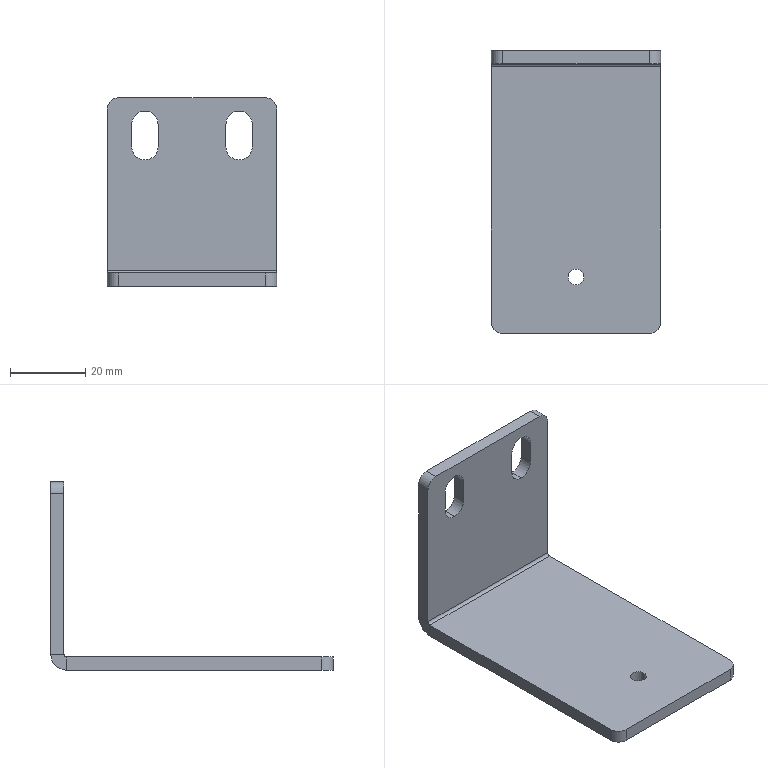Part | SolidWorks | features HoleWzd 2, EdgeFlange 1, Fillet 1, FlatPattern 1, ICE 1, MirrorPattern 1, SMBaseFlange 1, SheetMetal 1 | 1 solid | 30 faces | box 45 x 75 x 50 mm | volume 18329 mm3 | plane 16 | cylinder 14 | commonest cylinder face diameters 7 x6 6 x4 4.2 x2 1.473 x1 8.473 x1
STEP:
#1=CARTESIAN_POINT('',(16.,37.5,33.5));
#2=VERTEX_POINT('',#1);
#3=CARTESIAN_POINT('',(12.5,37.5,30.));
#4=VERTEX_POINT('',#3);
#5=CARTESIAN_POINT('',(12.5,37.5,33.5));
#6=DIRECTION('',(0.,1.,0.));
#7=DIRECTION('',(0.,0.,-1.));
#8=AXIS2_PLACEMENT_3D('',#5,#6,#7);
#9=CIRCLE('',#8,3.5);
#10=EDGE_CURVE('',#2,#4,#9,.T.);
#11=ORIENTED_EDGE('',*,*,#10,.T.);
#12=CARTESIAN_POINT('',(12.5,34.,30.));
#13=VERTEX_POINT('',#12);
#14=CARTESIAN_POINT('',(12.5,37.5,30.));
#15=DIRECTION('',(0.,-1.,0.));
#16=VECTOR('',#15,1000.);
#17=LINE('',#14,#16);
#18=EDGE_CURVE('',#4,#13,#17,.T.);
#19=ORIENTED_EDGE('',*,*,#18,.T.);
#20=CARTESIAN_POINT('',(16.,34.,33.5));
#21=VERTEX_POINT('',#20);
#22=CARTESIAN_POINT('',(12.5,34.,33.5));
#23=DIRECTION('',(0.,1.,0.));
#24=DIRECTION('',(0.,0.,-1.));
#25=AXIS2_PLACEMENT_3D('',#22,#23,#24);
#26=CIRCLE('',#25,3.5);
#27=EDGE_CURVE('',#21,#13,#26,.T.);
#28=ORIENTED_EDGE('',*,*,#27,.F.);
#29=CARTESIAN_POINT('',(16.,37.5,33.5));
#30=DIRECTION('',(0.,-1.,0.));
#31=VECTOR('',#30,1000.);
#32=LINE('',#29,#31);
#33=EDGE_CURVE('',#2,#21,#32,.T.);
#34=ORIENTED_EDGE('',*,*,#33,.F.);
#35=EDGE_LOOP('',(#11,#19,#28,#34));
#36=FACE_OUTER_BOUND('',#35,.T.);
#37=CARTESIAN_POINT('',(12.5,37.5,33.5));
#38=DIRECTION('',(0.,-1.,0.));
#39=DIRECTION('',(0.,0.,-1.));
#40=AXIS2_PLACEMENT_3D('',#37,#38,#39);
#41=CYLINDRICAL_SURFACE('',#40,3.5);
#42=ADVANCED_FACE('',(#36),#41,.F.);
#43=CARTESIAN_POINT('',(-12.5,37.5,30.));
#44=VERTEX_POINT('',#43);
#45=CARTESIAN_POINT('',(-9.,37.5,33.5));
#46=VERTEX_POINT('',#45);
#47=CARTESIAN_POINT('',(-12.5,37.5,33.5));
#48=DIRECTION('',(0.,-1.,0.));
#49=DIRECTION('',(0.,0.,-1.));
#50=AXIS2_PLACEMENT_3D('',#47,#48,#49);
#51=CIRCLE('',#50,3.5);
#52=EDGE_CURVE('',#44,#46,#51,.T.);
#53=ORIENTED_EDGE('',*,*,#52,.F.);
#54=CARTESIAN_POINT('',(-12.5,34.,30.));
#55=VERTEX_POINT('',#54);
#56=CARTESIAN_POINT('',(-12.5,37.5,30.));
#57=DIRECTION('',(0.,-1.,0.));
#58=VECTOR('',#57,1000.);
#59=LINE('',#56,#58);
#60=EDGE_CURVE('',#44,#55,#59,.T.);
#61=ORIENTED_EDGE('',*,*,#60,.T.);
#62=CARTESIAN_POINT('',(-9.,34.,33.5));
#63=VERTEX_POINT('',#62);
#64=CARTESIAN_POINT('',(-12.5,34.,33.5));
#65=DIRECTION('',(0.,-1.,0.));
#66=DIRECTION('',(0.,0.,-1.));
#67=AXIS2_PLACEMENT_3D('',#64,#65,#66);
#68=CIRCLE('',#67,3.5);
#69=EDGE_CURVE('',#55,#63,#68,.T.);
#70=ORIENTED_EDGE('',*,*,#69,.T.);
#71=CARTESIAN_POINT('',(-9.,37.5,33.5));
#72=DIRECTION('',(0.,-1.,0.));
#73=VECTOR('',#72,1000.);
#74=LINE('',#71,#73);
#75=EDGE_CURVE('',#46,#63,#74,.T.);
#76=ORIENTED_EDGE('',*,*,#75,.F.);
#77=EDGE_LOOP('',(#53,#61,#70,#76));
#78=FACE_OUTER_BOUND('',#77,.T.);
#79=CARTESIAN_POINT('',(-12.5,37.5,33.5));
#80=DIRECTION('',(0.,-1.,0.));
#81=DIRECTION('',(0.,0.,-1.));
#82=AXIS2_PLACEMENT_3D('',#79,#80,#81);
#83=CYLINDRICAL_SURFACE('',#82,3.5);
#84=ADVANCED_FACE('',(#78),#83,.F.);
#85=CARTESIAN_POINT('',(-2.1,-22.5,-3.5));
#86=VERTEX_POINT('',#85);
#87=CARTESIAN_POINT('',(2.1,-22.5,-3.5));
#88=VERTEX_POINT('',#87);
#89=CARTESIAN_POINT('',(0.,-22.5,-3.5));
#90=DIRECTION('',(0.,0.,1.));
#91=DIRECTION('',(1.,0.,0.));
#92=AXIS2_PLACEMENT_3D('',#89,#90,#91);
#93=CIRCLE('',#92,2.1);
#94=EDGE_CURVE('',#86,#88,#93,.T.);
#95=ORIENTED_EDGE('',*,*,#94,.F.);
#96=CARTESIAN_POINT('',(-2.1,-22.5,0.));
#97=VERTEX_POINT('',#96);
#98=CARTESIAN_POINT('',(-2.1,-22.5,0.));
#99=DIRECTION('',(0.,0.,1.));
#100=VECTOR('',#99,1000.);
#101=LINE('',#98,#100);
#102=EDGE_CURVE('',#86,#97,#101,.T.);
#103=ORIENTED_EDGE('',*,*,#102,.T.);
#104=CARTESIAN_POINT('',(2.1,-22.5,0.));
#105=VERTEX_POINT('',#104);
#106=CARTESIAN_POINT('',(0.,-22.5,0.));
#107=DIRECTION('',(0.,0.,1.));
#108=DIRECTION('',(1.,0.,0.));
#109=AXIS2_PLACEMENT_3D('',#106,#107,#108);
#110=CIRCLE('',#109,2.1);
#111=EDGE_CURVE('',#97,#105,#110,.T.);
#112=ORIENTED_EDGE('',*,*,#111,.T.);
#113=CARTESIAN_POINT('',(2.1,-22.5,0.));
#114=DIRECTION('',(0.,0.,1.));
#115=VECTOR('',#114,1000.);
#116=LINE('',#113,#115);
#117=EDGE_CURVE('',#88,#105,#116,.T.);
#118=ORIENTED_EDGE('',*,*,#117,.F.);
#119=EDGE_LOOP('',(#95,#103,#112,#118));
#120=FACE_OUTER_BOUND('',#119,.T.);
#121=CARTESIAN_POINT('',(0.,-22.5,0.));
#122=DIRECTION('',(0.,0.,1.));
#123=DIRECTION('',(1.,0.,0.));
#124=AXIS2_PLACEMENT_3D('',#121,#122,#123);
#125=CYLINDRICAL_SURFACE('',#124,2.1);
#126=ADVANCED_FACE('',(#120),#125,.F.);
#127=CARTESIAN_POINT('',(-16.,37.5,33.5));
#128=VERTEX_POINT('',#127);
#129=CARTESIAN_POINT('',(-12.5,37.5,33.5));
#130=DIRECTION('',(0.,-1.,0.));
#131=DIRECTION('',(0.,0.,-1.));
#132=AXIS2_PLACEMENT_3D('',#129,#130,#131);
#133=CIRCLE('',#132,3.5);
#134=EDGE_CURVE('',#128,#44,#133,.T.);
#135=ORIENTED_EDGE('',*,*,#134,.T.);
#136=ORIENTED_EDGE('',*,*,#52,.T.);
#137=CARTESIAN_POINT('',(-9.,37.5,39.5));
#138=VERTEX_POINT('',#137);
#139=CARTESIAN_POINT('',(-9.,37.5,39.5));
#140=DIRECTION('',(0.,0.,1.));
#141=VECTOR('',#140,1000.);
#142=LINE('',#139,#141);
#143=EDGE_CURVE('',#46,#138,#142,.T.);
#144=ORIENTED_EDGE('',*,*,#143,.T.);
#145=CARTESIAN_POINT('',(-16.,37.5,39.5));
#146=VERTEX_POINT('',#145);
#147=CARTESIAN_POINT('',(-12.5,37.5,39.5));
#148=DIRECTION('',(0.,-1.,0.));
#149=DIRECTION('',(0.,0.,-1.));
#150=AXIS2_PLACEMENT_3D('',#147,#148,#149);
#151=CIRCLE('',#150,3.5);
#152=EDGE_CURVE('',#138,#146,#151,.T.);
#153=ORIENTED_EDGE('',*,*,#152,.T.);
#154=CARTESIAN_POINT('',(-16.,37.5,39.5));
#155=DIRECTION('',(0.,0.,-1.));
#156=VECTOR('',#155,1000.);
#157=LINE('',#154,#156);
#158=EDGE_CURVE('',#146,#128,#157,.T.);
#159=ORIENTED_EDGE('',*,*,#158,.T.);
#160=EDGE_LOOP('',(#135,#136,#144,#153,#159));
#161=FACE_BOUND('',#160,.T.);
#162=CARTESIAN_POINT('',(-19.5,37.5,46.5));
#163=VERTEX_POINT('',#162);
#164=CARTESIAN_POINT('',(19.5,37.5,46.5));
#165=VERTEX_POINT('',#164);
#166=CARTESIAN_POINT('',(0.,37.5,46.5));
#167=DIRECTION('',(1.,0.,0.));
#168=VECTOR('',#167,1000.);
#169=LINE('',#166,#168);
#170=EDGE_CURVE('',#163,#165,#169,.T.);
#171=ORIENTED_EDGE('',*,*,#170,.T.);
#172=CARTESIAN_POINT('',(22.5,37.5,43.5));
#173=VERTEX_POINT('',#172);
#174=CARTESIAN_POINT('',(19.5,37.5,43.5));
#175=DIRECTION('',(0.,1.,0.));
#176=DIRECTION('',(0.,0.,-1.));
#177=AXIS2_PLACEMENT_3D('',#174,#175,#176);
#178=CIRCLE('',#177,3.);
#179=EDGE_CURVE('',#165,#173,#178,.T.);
#180=ORIENTED_EDGE('',*,*,#179,.T.);
#181=CARTESIAN_POINT('',(22.5,37.5,0.7366));
#182=VERTEX_POINT('',#181);
#183=CARTESIAN_POINT('',(22.5,37.5,0.));
#184=DIRECTION('',(0.,0.,-1.));
#185=VECTOR('',#184,1000.);
#186=LINE('',#183,#185);
#187=EDGE_CURVE('',#173,#182,#186,.T.);
#188=ORIENTED_EDGE('',*,*,#187,.T.);
#189=CARTESIAN_POINT('',(-22.5,37.5,0.7366));
#190=VERTEX_POINT('',#189);
#191=CARTESIAN_POINT('',(22.5,37.5,0.7366));
#192=DIRECTION('',(1.,0.,0.));
#193=VECTOR('',#192,1000.);
#194=LINE('',#191,#193);
#195=EDGE_CURVE('',#190,#182,#194,.T.);
#196=ORIENTED_EDGE('',*,*,#195,.F.);
#197=CARTESIAN_POINT('',(-22.5,37.5,43.5));
#198=VERTEX_POINT('',#197);
#199=CARTESIAN_POINT('',(-22.5,37.5,0.));
#200=DIRECTION('',(0.,0.,1.));
#201=VECTOR('',#200,1000.);
#202=LINE('',#199,#201);
#203=EDGE_CURVE('',#190,#198,#202,.T.);
#204=ORIENTED_EDGE('',*,*,#203,.T.);
#205=CARTESIAN_POINT('',(-19.5,37.5,43.5));
#206=DIRECTION('',(0.,1.,0.));
#207=DIRECTION('',(0.,0.,-1.));
#208=AXIS2_PLACEMENT_3D('',#205,#206,#207);
#209=CIRCLE('',#208,3.);
#210=EDGE_CURVE('',#198,#163,#209,.T.);
#211=ORIENTED_EDGE('',*,*,#210,.T.);
#212=EDGE_LOOP('',(#171,#180,#188,#196,#204,#211));
#213=FACE_OUTER_BOUND('',#212,.T.);
#214=CARTESIAN_POINT('',(9.,37.5,39.5));
#215=VERTEX_POINT('',#214);
#216=CARTESIAN_POINT('',(16.,37.5,39.5));
#217=VERTEX_POINT('',#216);
#218=CARTESIAN_POINT('',(12.5,37.5,39.5));
#219=DIRECTION('',(0.,1.,0.));
#220=DIRECTION('',(0.,0.,-1.));
#221=AXIS2_PLACEMENT_3D('',#218,#219,#220);
#222=CIRCLE('',#221,3.5);
#223=EDGE_CURVE('',#215,#217,#222,.T.);
#224=ORIENTED_EDGE('',*,*,#223,.F.);
#225=CARTESIAN_POINT('',(9.,37.5,33.5));
#226=VERTEX_POINT('',#225);
#227=CARTESIAN_POINT('',(9.,37.5,39.5));
#228=DIRECTION('',(0.,0.,1.));
#229=VECTOR('',#228,1000.);
#230=LINE('',#227,#229);
#231=EDGE_CURVE('',#226,#215,#230,.T.);
#232=ORIENTED_EDGE('',*,*,#231,.F.);
#233=CARTESIAN_POINT('',(12.5,37.5,33.5));
#234=DIRECTION('',(0.,1.,0.));
#235=DIRECTION('',(0.,0.,-1.));
#236=AXIS2_PLACEMENT_3D('',#233,#234,#235);
#237=CIRCLE('',#236,3.5);
#238=EDGE_CURVE('',#4,#226,#237,.T.);
#239=ORIENTED_EDGE('',*,*,#238,.F.);
#240=ORIENTED_EDGE('',*,*,#10,.F.);
#241=CARTESIAN_POINT('',(16.,37.5,39.5));
#242=DIRECTION('',(0.,0.,-1.));
#243=VECTOR('',#242,1000.);
#244=LINE('',#241,#243);
#245=EDGE_CURVE('',#217,#2,#244,.T.);
#246=ORIENTED_EDGE('',*,*,#245,.F.);
#247=EDGE_LOOP('',(#224,#232,#239,#240,#246));
#248=FACE_BOUND('',#247,.T.);
#249=CARTESIAN_POINT('',(0.,37.5,0.));
#250=DIRECTION('',(0.,-1.,0.));
#251=DIRECTION('',(0.,0.,-1.));
#252=AXIS2_PLACEMENT_3D('',#249,#250,#251);
#253=PLANE('',#252);
#254=ADVANCED_FACE('',(#161,#213,#248),#253,.F.);
#255=CARTESIAN_POINT('',(-9.,34.,39.5));
#256=VERTEX_POINT('',#255);
#257=CARTESIAN_POINT('',(-9.,34.,39.5));
#258=DIRECTION('',(0.,0.,1.));
#259=VECTOR('',#258,1000.);
#260=LINE('',#257,#259);
#261=EDGE_CURVE('',#63,#256,#260,.T.);
#262=ORIENTED_EDGE('',*,*,#261,.F.);
#263=ORIENTED_EDGE('',*,*,#69,.F.);
#264=CARTESIAN_POINT('',(-16.,34.,33.5));
#265=VERTEX_POINT('',#264);
#266=CARTESIAN_POINT('',(-12.5,34.,33.5));
#267=DIRECTION('',(0.,-1.,0.));
#268=DIRECTION('',(0.,0.,-1.));
#269=AXIS2_PLACEMENT_3D('',#266,#267,#268);
#270=CIRCLE('',#269,3.5);
#271=EDGE_CURVE('',#265,#55,#270,.T.);
#272=ORIENTED_EDGE('',*,*,#271,.F.);
#273=CARTESIAN_POINT('',(-16.,34.,39.5));
#274=VERTEX_POINT('',#273);
#275=CARTESIAN_POINT('',(-16.,34.,39.5));
#276=DIRECTION('',(0.,0.,-1.));
#277=VECTOR('',#276,1000.);
#278=LINE('',#275,#277);
#279=EDGE_CURVE('',#274,#265,#278,.T.);
#280=ORIENTED_EDGE('',*,*,#279,.F.);
#281=CARTESIAN_POINT('',(-12.5,34.,39.5));
#282=DIRECTION('',(0.,-1.,0.));
#283=DIRECTION('',(0.,0.,-1.));
#284=AXIS2_PLACEMENT_3D('',#281,#282,#283);
#285=CIRCLE('',#284,3.5);
#286=EDGE_CURVE('',#256,#274,#285,.T.);
#287=ORIENTED_EDGE('',*,*,#286,.F.);
#288=EDGE_LOOP('',(#262,#263,#272,#280,#287));
#289=FACE_BOUND('',#288,.T.);
#290=CARTESIAN_POINT('',(22.5,34.,43.5));
#291=VERTEX_POINT('',#290);
#292=CARTESIAN_POINT('',(22.5,34.,0.7366));
#293=VERTEX_POINT('',#292);
#294=CARTESIAN_POINT('',(22.5,34.,0.));
#295=DIRECTION('',(0.,0.,-1.));
#296=VECTOR('',#295,1000.);
#297=LINE('',#294,#296);
#298=EDGE_CURVE('',#291,#293,#297,.T.);
#299=ORIENTED_EDGE('',*,*,#298,.F.);
#300=CARTESIAN_POINT('',(19.5,34.,46.5));
#301=VERTEX_POINT('',#300);
#302=CARTESIAN_POINT('',(19.5,34.,43.5));
#303=DIRECTION('',(0.,-1.,0.));
#304=DIRECTION('',(0.,0.,-1.));
#305=AXIS2_PLACEMENT_3D('',#302,#303,#304);
#306=CIRCLE('',#305,3.);
#307=EDGE_CURVE('',#291,#301,#306,.T.);
#308=ORIENTED_EDGE('',*,*,#307,.T.);
#309=CARTESIAN_POINT('',(-19.5,34.,46.5));
#310=VERTEX_POINT('',#309);
#311=CARTESIAN_POINT('',(22.5,34.,46.5));
#312=DIRECTION('',(1.,0.,0.));
#313=VECTOR('',#312,1000.);
#314=LINE('',#311,#313);
#315=EDGE_CURVE('',#310,#301,#314,.T.);
#316=ORIENTED_EDGE('',*,*,#315,.F.);
#317=CARTESIAN_POINT('',(-22.5,34.,43.5));
#318=VERTEX_POINT('',#317);
#319=CARTESIAN_POINT('',(-19.5,34.,43.5));
#320=DIRECTION('',(0.,-1.,0.));
#321=DIRECTION('',(0.,0.,-1.));
#322=AXIS2_PLACEMENT_3D('',#319,#320,#321);
#323=CIRCLE('',#322,3.);
#324=EDGE_CURVE('',#310,#318,#323,.T.);
#325=ORIENTED_EDGE('',*,*,#324,.T.);
#326=CARTESIAN_POINT('',(-22.5,34.,0.7366));
#327=VERTEX_POINT('',#326);
#328=CARTESIAN_POINT('',(-22.5,34.,46.5));
#329=DIRECTION('',(0.,0.,1.));
#330=VECTOR('',#329,1000.);
#331=LINE('',#328,#330);
#332=EDGE_CURVE('',#327,#318,#331,.T.);
#333=ORIENTED_EDGE('',*,*,#332,.F.);
#334=CARTESIAN_POINT('',(22.5,34.,0.7366));
#335=DIRECTION('',(-1.,0.,0.));
#336=VECTOR('',#335,1000.);
#337=LINE('',#334,#336);
#338=EDGE_CURVE('',#293,#327,#337,.T.);
#339=ORIENTED_EDGE('',*,*,#338,.F.);
#340=EDGE_LOOP('',(#299,#308,#316,#325,#333,#339));
#341=FACE_OUTER_BOUND('',#340,.T.);
#342=CARTESIAN_POINT('',(9.,34.,33.5));
#343=VERTEX_POINT('',#342);
#344=CARTESIAN_POINT('',(9.,34.,39.5));
#345=VERTEX_POINT('',#344);
#346=CARTESIAN_POINT('',(9.,34.,39.5));
#347=DIRECTION('',(0.,0.,1.));
#348=VECTOR('',#347,1000.);
#349=LINE('',#346,#348);
#350=EDGE_CURVE('',#343,#345,#349,.T.);
#351=ORIENTED_EDGE('',*,*,#350,.T.);
#352=CARTESIAN_POINT('',(16.,34.,39.5));
#353=VERTEX_POINT('',#352);
#354=CARTESIAN_POINT('',(12.5,34.,39.5));
#355=DIRECTION('',(0.,1.,0.));
#356=DIRECTION('',(0.,0.,-1.));
#357=AXIS2_PLACEMENT_3D('',#354,#355,#356);
#358=CIRCLE('',#357,3.5);
#359=EDGE_CURVE('',#345,#353,#358,.T.);
#360=ORIENTED_EDGE('',*,*,#359,.T.);
#361=CARTESIAN_POINT('',(16.,34.,39.5));
#362=DIRECTION('',(0.,0.,-1.));
#363=VECTOR('',#362,1000.);
#364=LINE('',#361,#363);
#365=EDGE_CURVE('',#353,#21,#364,.T.);
#366=ORIENTED_EDGE('',*,*,#365,.T.);
#367=ORIENTED_EDGE('',*,*,#27,.T.);
#368=CARTESIAN_POINT('',(12.5,34.,33.5));
#369=DIRECTION('',(0.,1.,0.));
#370=DIRECTION('',(0.,0.,-1.));
#371=AXIS2_PLACEMENT_3D('',#368,#369,#370);
#372=CIRCLE('',#371,3.5);
#373=EDGE_CURVE('',#13,#343,#372,.T.);
#374=ORIENTED_EDGE('',*,*,#373,.T.);
#375=EDGE_LOOP('',(#351,#360,#366,#367,#374));
#376=FACE_BOUND('',#375,.T.);
#377=CARTESIAN_POINT('',(0.,34.,0.));
#378=DIRECTION('',(0.,-1.,0.));
#379=DIRECTION('',(0.,0.,-1.));
#380=AXIS2_PLACEMENT_3D('',#377,#378,#379);
#381=PLANE('',#380);
#382=ADVANCED_FACE('',(#289,#341,#376),#381,.T.);
#383=CARTESIAN_POINT('',(-22.5,33.263,-3.5));
#384=VERTEX_POINT('',#383);
#385=CARTESIAN_POINT('',(-22.5,-34.5,-3.5));
#386=VERTEX_POINT('',#385);
#387=CARTESIAN_POINT('',(-22.5,37.5,-3.5));
#388=DIRECTION('',(0.,-1.,0.));
#389=VECTOR('',#388,1000.);
#390=LINE('',#387,#389);
#391=EDGE_CURVE('',#384,#386,#390,.T.);
#392=ORIENTED_EDGE('',*,*,#391,.T.);
#393=CARTESIAN_POINT('',(-22.5,-34.5,0.));
#394=VERTEX_POINT('',#393);
#395=CARTESIAN_POINT('',(-22.5,-34.5,-3.5));
#396=DIRECTION('',(0.,0.,1.));
#397=VECTOR('',#396,1000.);
#398=LINE('',#395,#397);
#399=EDGE_CURVE('',#386,#394,#398,.T.);
#400=ORIENTED_EDGE('',*,*,#399,.T.);
#401=CARTESIAN_POINT('',(-22.5,33.263,0.));
#402=VERTEX_POINT('',#401);
#403=CARTESIAN_POINT('',(-22.5,37.5,0.));
#404=DIRECTION('',(0.,-1.,0.));
#405=VECTOR('',#404,1000.);
#406=LINE('',#403,#405);
#407=EDGE_CURVE('',#402,#394,#406,.T.);
#408=ORIENTED_EDGE('',*,*,#407,.F.);
#409=CARTESIAN_POINT('',(-22.5,33.263,0.));
#410=DIRECTION('',(0.,0.,-1.));
#411=VECTOR('',#410,1000.);
#412=LINE('',#409,#411);
#413=EDGE_CURVE('',#402,#384,#412,.T.);
#414=ORIENTED_EDGE('',*,*,#413,.T.);
#415=EDGE_LOOP('',(#392,#400,#408,#414));
#416=FACE_OUTER_BOUND('',#415,.T.);
#417=CARTESIAN_POINT('',(-22.5,37.5,-3.5));
#418=DIRECTION('',(-1.,0.,0.));
#419=DIRECTION('',(0.,-1.,0.));
#420=AXIS2_PLACEMENT_3D('',#417,#418,#419);
#421=PLANE('',#420);
#422=ADVANCED_FACE('',(#416),#421,.T.);
#423=CARTESIAN_POINT('',(0.,-22.5,-3.5));
#424=DIRECTION('',(0.,0.,1.));
#425=DIRECTION('',(1.,0.,0.));
#426=AXIS2_PLACEMENT_3D('',#423,#424,#425);
#427=CIRCLE('',#426,2.1);
#428=EDGE_CURVE('',#88,#86,#427,.T.);
#429=ORIENTED_EDGE('',*,*,#428,.T.);
#430=ORIENTED_EDGE('',*,*,#94,.T.);
#431=EDGE_LOOP('',(#429,#430));
#432=FACE_BOUND('',#431,.T.);
#433=CARTESIAN_POINT('',(-19.5,-37.5,-3.5));
#434=VERTEX_POINT('',#433);
#435=CARTESIAN_POINT('',(19.5,-37.5,-3.5));
#436=VERTEX_POINT('',#435);
#437=CARTESIAN_POINT('',(-22.5,-37.5,-3.5));
#438=DIRECTION('',(1.,0.,0.));
#439=VECTOR('',#438,1000.);
#440=LINE('',#437,#439);
#441=EDGE_CURVE('',#434,#436,#440,.T.);
#442=ORIENTED_EDGE('',*,*,#441,.F.);
#443=CARTESIAN_POINT('',(-19.5,-34.5,-3.5));
#444=DIRECTION('',(0.,0.,-1.));
#445=DIRECTION('',(1.,0.,0.));
#446=AXIS2_PLACEMENT_3D('',#443,#444,#445);
#447=CIRCLE('',#446,3.);
#448=EDGE_CURVE('',#434,#386,#447,.T.);
#449=ORIENTED_EDGE('',*,*,#448,.T.);
#450=ORIENTED_EDGE('',*,*,#391,.F.);
#451=CARTESIAN_POINT('',(22.5,33.263,-3.5));
#452=VERTEX_POINT('',#451);
#453=CARTESIAN_POINT('',(-22.5,33.263,-3.5));
#454=DIRECTION('',(1.,0.,0.));
#455=VECTOR('',#454,1000.);
#456=LINE('',#453,#455);
#457=EDGE_CURVE('',#384,#452,#456,.T.);
#458=ORIENTED_EDGE('',*,*,#457,.T.);
#459=CARTESIAN_POINT('',(22.5,-34.5,-3.5));
#460=VERTEX_POINT('',#459);
#461=CARTESIAN_POINT('',(22.5,37.5,-3.5));
#462=DIRECTION('',(0.,1.,0.));
#463=VECTOR('',#462,1000.);
#464=LINE('',#461,#463);
#465=EDGE_CURVE('',#460,#452,#464,.T.);
#466=ORIENTED_EDGE('',*,*,#465,.F.);
#467=CARTESIAN_POINT('',(19.5,-34.5,-3.5));
#468=DIRECTION('',(0.,0.,-1.));
#469=DIRECTION('',(1.,0.,0.));
#470=AXIS2_PLACEMENT_3D('',#467,#468,#469);
#471=CIRCLE('',#470,3.);
#472=EDGE_CURVE('',#460,#436,#471,.T.);
#473=ORIENTED_EDGE('',*,*,#472,.T.);
#474=EDGE_LOOP('',(#442,#449,#450,#458,#466,#473));
#475=FACE_OUTER_BOUND('',#474,.T.);
#476=CARTESIAN_POINT('',(0.,0.,-3.5));
#477=DIRECTION('',(0.,0.,1.));
#478=DIRECTION('',(1.,0.,0.));
#479=AXIS2_PLACEMENT_3D('',#476,#477,#478);
#480=PLANE('',#479);
#481=ADVANCED_FACE('',(#432,#475),#480,.F.);
#482=CARTESIAN_POINT('',(0.,-22.5,0.));
#483=DIRECTION('',(0.,0.,1.));
#484=DIRECTION('',(1.,0.,0.));
#485=AXIS2_PLACEMENT_3D('',#482,#483,#484);
#486=CIRCLE('',#485,2.1);
#487=EDGE_CURVE('',#105,#97,#486,.T.);
#488=ORIENTED_EDGE('',*,*,#487,.F.);
#489=ORIENTED_EDGE('',*,*,#111,.F.);
#490=EDGE_LOOP('',(#488,#489));
#491=FACE_BOUND('',#490,.T.);
#492=ORIENTED_EDGE('',*,*,#407,.T.);
#493=CARTESIAN_POINT('',(-19.5,-37.5,0.));
#494=VERTEX_POINT('',#493);
#495=CARTESIAN_POINT('',(-19.5,-34.5,0.));
#496=DIRECTION('',(0.,0.,1.));
#497=DIRECTION('',(1.,0.,0.));
#498=AXIS2_PLACEMENT_3D('',#495,#496,#497);
#499=CIRCLE('',#498,3.);
#500=EDGE_CURVE('',#394,#494,#499,.T.);
#501=ORIENTED_EDGE('',*,*,#500,.T.);
#502=CARTESIAN_POINT('',(19.5,-37.5,0.));
#503=VERTEX_POINT('',#502);
#504=CARTESIAN_POINT('',(-22.5,-37.5,0.));
#505=DIRECTION('',(1.,0.,0.));
#506=VECTOR('',#505,1000.);
#507=LINE('',#504,#506);
#508=EDGE_CURVE('',#494,#503,#507,.T.);
#509=ORIENTED_EDGE('',*,*,#508,.T.);
#510=CARTESIAN_POINT('',(22.5,-34.5,0.));
#511=VERTEX_POINT('',#510);
#512=CARTESIAN_POINT('',(19.5,-34.5,0.));
#513=DIRECTION('',(0.,0.,1.));
#514=DIRECTION('',(1.,0.,0.));
#515=AXIS2_PLACEMENT_3D('',#512,#513,#514);
#516=CIRCLE('',#515,3.);
#517=EDGE_CURVE('',#503,#511,#516,.T.);
#518=ORIENTED_EDGE('',*,*,#517,.T.);
#519=CARTESIAN_POINT('',(22.5,33.263,0.));
#520=VERTEX_POINT('',#519);
#521=CARTESIAN_POINT('',(22.5,37.5,0.));
#522=DIRECTION('',(0.,1.,0.));
#523=VECTOR('',#522,1000.);
#524=LINE('',#521,#523);
#525=EDGE_CURVE('',#511,#520,#524,.T.);
#526=ORIENTED_EDGE('',*,*,#525,.T.);
#527=CARTESIAN_POINT('',(-22.5,33.263,0.));
#528=DIRECTION('',(1.,0.,0.));
#529=VECTOR('',#528,1000.);
#530=LINE('',#527,#529);
#531=EDGE_CURVE('',#402,#520,#530,.T.);
#532=ORIENTED_EDGE('',*,*,#531,.F.);
#533=EDGE_LOOP('',(#492,#501,#509,#518,#526,#532));
#534=FACE_OUTER_BOUND('',#533,.T.);
#535=CARTESIAN_POINT('',(0.,0.,0.));
#536=DIRECTION('',(0.,0.,1.));
#537=DIRECTION('',(1.,0.,0.));
#538=AXIS2_PLACEMENT_3D('',#535,#536,#537);
#539=PLANE('',#538);
#540=ADVANCED_FACE('',(#491,#534),#539,.T.);
#541=ORIENTED_EDGE('',*,*,#525,.F.);
#542=CARTESIAN_POINT('',(22.5,-34.5,-3.5));
#543=DIRECTION('',(0.,0.,-1.));
#544=VECTOR('',#543,1000.);
#545=LINE('',#542,#544);
#546=EDGE_CURVE('',#511,#460,#545,.T.);
#547=ORIENTED_EDGE('',*,*,#546,.T.);
#548=ORIENTED_EDGE('',*,*,#465,.T.);
#549=CARTESIAN_POINT('',(22.5,33.263,0.));
#550=DIRECTION('',(0.,0.,-1.));
#551=VECTOR('',#550,1000.);
#552=LINE('',#549,#551);
#553=EDGE_CURVE('',#520,#452,#552,.T.);
#554=ORIENTED_EDGE('',*,*,#553,.F.);
#555=EDGE_LOOP('',(#541,#547,#548,#554));
#556=FACE_OUTER_BOUND('',#555,.T.);
#557=CARTESIAN_POINT('',(22.5,37.5,-3.5));
#558=DIRECTION('',(1.,0.,0.));
#559=DIRECTION('',(0.,1.,0.));
#560=AXIS2_PLACEMENT_3D('',#557,#558,#559);
#561=PLANE('',#560);
#562=ADVANCED_FACE('',(#556),#561,.T.);
#563=ORIENTED_EDGE('',*,*,#508,.F.);
#564=CARTESIAN_POINT('',(-19.5,-37.5,-3.5));
#565=DIRECTION('',(0.,0.,-1.));
#566=VECTOR('',#565,1000.);
#567=LINE('',#564,#566);
#568=EDGE_CURVE('',#494,#434,#567,.T.);
#569=ORIENTED_EDGE('',*,*,#568,.T.);
#570=ORIENTED_EDGE('',*,*,#441,.T.);
#571=CARTESIAN_POINT('',(19.5,-37.5,-3.5));
#572=DIRECTION('',(0.,0.,1.));
#573=VECTOR('',#572,1000.);
#574=LINE('',#571,#573);
#575=EDGE_CURVE('',#436,#503,#574,.T.);
#576=ORIENTED_EDGE('',*,*,#575,.T.);
#577=EDGE_LOOP('',(#563,#569,#570,#576));
#578=FACE_OUTER_BOUND('',#577,.T.);
#579=CARTESIAN_POINT('',(-22.5,-37.5,-3.5));
#580=DIRECTION('',(0.,-1.,0.));
#581=DIRECTION('',(0.,0.,-1.));
#582=AXIS2_PLACEMENT_3D('',#579,#580,#581);
#583=PLANE('',#582);
#584=ADVANCED_FACE('',(#578),#583,.T.);
#585=CARTESIAN_POINT('',(22.5,37.5,0.7366));
#586=DIRECTION('',(0.,1.,0.));
#587=VECTOR('',#586,1000.);
#588=LINE('',#585,#587);
#589=EDGE_CURVE('',#293,#182,#588,.T.);
#590=ORIENTED_EDGE('',*,*,#589,.F.);
#591=CARTESIAN_POINT('',(22.5,33.263,0.7366));
#592=DIRECTION('',(1.,0.,0.));
#593=DIRECTION('',(0.,0.,1.));
#594=AXIS2_PLACEMENT_3D('',#591,#592,#593);
#595=CIRCLE('',#594,0.7366);
#596=EDGE_CURVE('',#520,#293,#595,.T.);
#597=ORIENTED_EDGE('',*,*,#596,.F.);
#598=ORIENTED_EDGE('',*,*,#553,.T.);
#599=CARTESIAN_POINT('',(22.5,33.263,0.7366));
#600=DIRECTION('',(1.,0.,0.));
#601=DIRECTION('',(0.,0.,1.));
#602=AXIS2_PLACEMENT_3D('',#599,#600,#601);
#603=CIRCLE('',#602,4.237);
#604=EDGE_CURVE('',#452,#182,#603,.T.);
#605=ORIENTED_EDGE('',*,*,#604,.T.);
#606=EDGE_LOOP('',(#590,#597,#598,#605));
#607=FACE_OUTER_BOUND('',#606,.T.);
#608=CARTESIAN_POINT('',(22.5,33.263,0.7366));
#609=DIRECTION('',(1.,0.,0.));
#610=DIRECTION('',(0.,0.,-1.));
#611=AXIS2_PLACEMENT_3D('',#608,#609,#610);
#612=PLANE('',#611);
#613=ADVANCED_FACE('',(#607),#612,.T.);
#614=CARTESIAN_POINT('',(-22.5,33.263,0.7366));
#615=DIRECTION('',(-1.,0.,0.));
#616=DIRECTION('',(0.,0.,1.));
#617=AXIS2_PLACEMENT_3D('',#614,#615,#616);
#618=CIRCLE('',#617,0.7366);
#619=EDGE_CURVE('',#327,#402,#618,.T.);
#620=ORIENTED_EDGE('',*,*,#619,.F.);
#621=CARTESIAN_POINT('',(-22.5,34.,0.7366));
#622=DIRECTION('',(0.,1.,0.));
#623=VECTOR('',#622,1000.);
#624=LINE('',#621,#623);
#625=EDGE_CURVE('',#327,#190,#624,.T.);
#626=ORIENTED_EDGE('',*,*,#625,.T.);
#627=CARTESIAN_POINT('',(-22.5,33.263,0.7366));
#628=DIRECTION('',(-1.,0.,0.));
#629=DIRECTION('',(0.,0.,1.));
#630=AXIS2_PLACEMENT_3D('',#627,#628,#629);
#631=CIRCLE('',#630,4.237);
#632=EDGE_CURVE('',#190,#384,#631,.T.);
#633=ORIENTED_EDGE('',*,*,#632,.T.);
#634=ORIENTED_EDGE('',*,*,#413,.F.);
#635=EDGE_LOOP('',(#620,#626,#633,#634));
#636=FACE_OUTER_BOUND('',#635,.T.);
#637=CARTESIAN_POINT('',(-22.5,33.263,0.7366));
#638=DIRECTION('',(1.,0.,0.));
#639=DIRECTION('',(0.,0.,-1.));
#640=AXIS2_PLACEMENT_3D('',#637,#638,#639);
#641=PLANE('',#640);
#642=ADVANCED_FACE('',(#636),#641,.F.);
#643=ORIENTED_EDGE('',*,*,#457,.F.);
#644=ORIENTED_EDGE('',*,*,#632,.F.);
#645=ORIENTED_EDGE('',*,*,#195,.T.);
#646=ORIENTED_EDGE('',*,*,#604,.F.);
#647=EDGE_LOOP('',(#643,#644,#645,#646));
#648=FACE_OUTER_BOUND('',#647,.T.);
#649=CARTESIAN_POINT('',(-22.5,33.263,0.7366));
#650=DIRECTION('',(-1.,0.,0.));
#651=DIRECTION('',(0.,1.,0.));
#652=AXIS2_PLACEMENT_3D('',#649,#650,#651);
#653=CYLINDRICAL_SURFACE('',#652,4.237);
#654=ADVANCED_FACE('',(#648),#653,.T.);
#655=ORIENTED_EDGE('',*,*,#531,.T.);
#656=ORIENTED_EDGE('',*,*,#596,.T.);
#657=ORIENTED_EDGE('',*,*,#338,.T.);
#658=ORIENTED_EDGE('',*,*,#619,.T.);
#659=EDGE_LOOP('',(#655,#656,#657,#658));
#660=FACE_OUTER_BOUND('',#659,.T.);
#661=CARTESIAN_POINT('',(-22.5,33.263,0.7366));
#662=DIRECTION('',(-1.,0.,0.));
#663=DIRECTION('',(0.,1.,0.));
#664=AXIS2_PLACEMENT_3D('',#661,#662,#663);
#665=CYLINDRICAL_SURFACE('',#664,0.7366);
#666=ADVANCED_FACE('',(#660),#665,.F.);
#667=ORIENTED_EDGE('',*,*,#187,.F.);
#668=CARTESIAN_POINT('',(22.5,37.5,43.5));
#669=DIRECTION('',(0.,-1.,0.));
#670=VECTOR('',#669,1000.);
#671=LINE('',#668,#670);
#672=EDGE_CURVE('',#173,#291,#671,.T.);
#673=ORIENTED_EDGE('',*,*,#672,.T.);
#674=ORIENTED_EDGE('',*,*,#298,.T.);
#675=ORIENTED_EDGE('',*,*,#589,.T.);
#676=EDGE_LOOP('',(#667,#673,#674,#675));
#677=FACE_OUTER_BOUND('',#676,.T.);
#678=CARTESIAN_POINT('',(22.5,37.5,0.));
#679=DIRECTION('',(-1.,0.,0.));
#680=DIRECTION('',(0.,0.,1.));
#681=AXIS2_PLACEMENT_3D('',#678,#679,#680);
#682=PLANE('',#681);
#683=ADVANCED_FACE('',(#677),#682,.F.);
#684=ORIENTED_EDGE('',*,*,#332,.T.);
#685=CARTESIAN_POINT('',(-22.5,37.5,43.5));
#686=DIRECTION('',(0.,1.,0.));
#687=VECTOR('',#686,1000.);
#688=LINE('',#685,#687);
#689=EDGE_CURVE('',#318,#198,#688,.T.);
#690=ORIENTED_EDGE('',*,*,#689,.T.);
#691=ORIENTED_EDGE('',*,*,#203,.F.);
#692=ORIENTED_EDGE('',*,*,#625,.F.);
#693=EDGE_LOOP('',(#684,#690,#691,#692));
#694=FACE_OUTER_BOUND('',#693,.T.);
#695=CARTESIAN_POINT('',(-22.5,37.5,46.5));
#696=DIRECTION('',(1.,0.,0.));
#697=DIRECTION('',(0.,0.,-1.));
#698=AXIS2_PLACEMENT_3D('',#695,#696,#697);
#699=PLANE('',#698);
#700=ADVANCED_FACE('',(#694),#699,.F.);
#701=ORIENTED_EDGE('',*,*,#315,.T.);
#702=CARTESIAN_POINT('',(19.5,37.5,46.5));
#703=DIRECTION('',(0.,1.,0.));
#704=VECTOR('',#703,1000.);
#705=LINE('',#702,#704);
#706=EDGE_CURVE('',#301,#165,#705,.T.);
#707=ORIENTED_EDGE('',*,*,#706,.T.);
#708=ORIENTED_EDGE('',*,*,#170,.F.);
#709=CARTESIAN_POINT('',(-19.5,37.5,46.5));
#710=DIRECTION('',(0.,-1.,0.));
#711=VECTOR('',#710,1000.);
#712=LINE('',#709,#711);
#713=EDGE_CURVE('',#163,#310,#712,.T.);
#714=ORIENTED_EDGE('',*,*,#713,.T.);
#715=EDGE_LOOP('',(#701,#707,#708,#714));
#716=FACE_OUTER_BOUND('',#715,.T.);
#717=CARTESIAN_POINT('',(22.5,37.5,46.5));
#718=DIRECTION('',(0.,0.,-1.));
#719=DIRECTION('',(0.,1.,0.));
#720=AXIS2_PLACEMENT_3D('',#717,#718,#719);
#721=PLANE('',#720);
#722=ADVANCED_FACE('',(#716),#721,.F.);
#723=ORIENTED_EDGE('',*,*,#102,.F.);
#724=ORIENTED_EDGE('',*,*,#428,.F.);
#725=ORIENTED_EDGE('',*,*,#117,.T.);
#726=ORIENTED_EDGE('',*,*,#487,.T.);
#727=EDGE_LOOP('',(#723,#724,#725,#726));
#728=FACE_OUTER_BOUND('',#727,.T.);
#729=CARTESIAN_POINT('',(0.,-22.5,0.));
#730=DIRECTION('',(0.,0.,1.));
#731=DIRECTION('',(1.,0.,0.));
#732=AXIS2_PLACEMENT_3D('',#729,#730,#731);
#733=CYLINDRICAL_SURFACE('',#732,2.1);
#734=ADVANCED_FACE('',(#728),#733,.F.);
#735=ORIENTED_EDGE('',*,*,#448,.F.);
#736=ORIENTED_EDGE('',*,*,#568,.F.);
#737=ORIENTED_EDGE('',*,*,#500,.F.);
#738=ORIENTED_EDGE('',*,*,#399,.F.);
#739=EDGE_LOOP('',(#735,#736,#737,#738));
#740=FACE_OUTER_BOUND('',#739,.T.);
#741=CARTESIAN_POINT('',(-19.5,-34.5,-3.5));
#742=DIRECTION('',(0.,0.,1.));
#743=DIRECTION('',(1.,0.,0.));
#744=AXIS2_PLACEMENT_3D('',#741,#742,#743);
#745=CYLINDRICAL_SURFACE('',#744,3.);
#746=ADVANCED_FACE('',(#740),#745,.T.);
#747=ORIENTED_EDGE('',*,*,#472,.F.);
#748=ORIENTED_EDGE('',*,*,#546,.F.);
#749=ORIENTED_EDGE('',*,*,#517,.F.);
#750=ORIENTED_EDGE('',*,*,#575,.F.);
#751=EDGE_LOOP('',(#747,#748,#749,#750));
#752=FACE_OUTER_BOUND('',#751,.T.);
#753=CARTESIAN_POINT('',(19.5,-34.5,-3.5));
#754=DIRECTION('',(0.,0.,1.));
#755=DIRECTION('',(1.,0.,0.));
#756=AXIS2_PLACEMENT_3D('',#753,#754,#755);
#757=CYLINDRICAL_SURFACE('',#756,3.);
#758=ADVANCED_FACE('',(#752),#757,.T.);
#759=ORIENTED_EDGE('',*,*,#179,.F.);
#760=ORIENTED_EDGE('',*,*,#706,.F.);
#761=ORIENTED_EDGE('',*,*,#307,.F.);
#762=ORIENTED_EDGE('',*,*,#672,.F.);
#763=EDGE_LOOP('',(#759,#760,#761,#762));
#764=FACE_OUTER_BOUND('',#763,.T.);
#765=CARTESIAN_POINT('',(19.5,37.5,43.5));
#766=DIRECTION('',(0.,-1.,0.));
#767=DIRECTION('',(0.,0.,-1.));
#768=AXIS2_PLACEMENT_3D('',#765,#766,#767);
#769=CYLINDRICAL_SURFACE('',#768,3.);
#770=ADVANCED_FACE('',(#764),#769,.T.);
#771=ORIENTED_EDGE('',*,*,#210,.F.);
#772=ORIENTED_EDGE('',*,*,#689,.F.);
#773=ORIENTED_EDGE('',*,*,#324,.F.);
#774=ORIENTED_EDGE('',*,*,#713,.F.);
#775=EDGE_LOOP('',(#771,#772,#773,#774));
#776=FACE_OUTER_BOUND('',#775,.T.);
#777=CARTESIAN_POINT('',(-19.5,37.5,43.5));
#778=DIRECTION('',(0.,-1.,0.));
#779=DIRECTION('',(0.,0.,-1.));
#780=AXIS2_PLACEMENT_3D('',#777,#778,#779);
#781=CYLINDRICAL_SURFACE('',#780,3.);
#782=ADVANCED_FACE('',(#776),#781,.T.);
#783=ORIENTED_EDGE('',*,*,#261,.T.);
#784=CARTESIAN_POINT('',(-9.,37.5,39.5));
#785=DIRECTION('',(0.,-1.,0.));
#786=VECTOR('',#785,1000.);
#787=LINE('',#784,#786);
#788=EDGE_CURVE('',#138,#256,#787,.T.);
#789=ORIENTED_EDGE('',*,*,#788,.F.);
#790=ORIENTED_EDGE('',*,*,#143,.F.);
#791=ORIENTED_EDGE('',*,*,#75,.T.);
#792=EDGE_LOOP('',(#783,#789,#790,#791));
#793=FACE_OUTER_BOUND('',#792,.T.);
#794=CARTESIAN_POINT('',(-9.,37.5,39.5));
#795=DIRECTION('',(1.,0.,0.));
#796=DIRECTION('',(0.,0.,-1.));
#797=AXIS2_PLACEMENT_3D('',#794,#795,#796);
#798=PLANE('',#797);
#799=ADVANCED_FACE('',(#793),#798,.F.);
#800=ORIENTED_EDGE('',*,*,#279,.T.);
#801=CARTESIAN_POINT('',(-16.,37.5,33.5));
#802=DIRECTION('',(0.,-1.,0.));
#803=VECTOR('',#802,1000.);
#804=LINE('',#801,#803);
#805=EDGE_CURVE('',#128,#265,#804,.T.);
#806=ORIENTED_EDGE('',*,*,#805,.F.);
#807=ORIENTED_EDGE('',*,*,#158,.F.);
#808=CARTESIAN_POINT('',(-16.,37.5,39.5));
#809=DIRECTION('',(0.,-1.,0.));
#810=VECTOR('',#809,1000.);
#811=LINE('',#808,#810);
#812=EDGE_CURVE('',#146,#274,#811,.T.);
#813=ORIENTED_EDGE('',*,*,#812,.T.);
#814=EDGE_LOOP('',(#800,#806,#807,#813));
#815=FACE_OUTER_BOUND('',#814,.T.);
#816=CARTESIAN_POINT('',(-16.,37.5,39.5));
#817=DIRECTION('',(-1.,0.,0.));
#818=DIRECTION('',(0.,0.,1.));
#819=AXIS2_PLACEMENT_3D('',#816,#817,#818);
#820=PLANE('',#819);
#821=ADVANCED_FACE('',(#815),#820,.F.);
#822=ORIENTED_EDGE('',*,*,#286,.T.);
#823=ORIENTED_EDGE('',*,*,#812,.F.);
#824=ORIENTED_EDGE('',*,*,#152,.F.);
#825=ORIENTED_EDGE('',*,*,#788,.T.);
#826=EDGE_LOOP('',(#822,#823,#824,#825));
#827=FACE_OUTER_BOUND('',#826,.T.);
#828=CARTESIAN_POINT('',(-12.5,37.5,39.5));
#829=DIRECTION('',(0.,-1.,0.));
#830=DIRECTION('',(0.,0.,-1.));
#831=AXIS2_PLACEMENT_3D('',#828,#829,#830);
#832=CYLINDRICAL_SURFACE('',#831,3.5);
#833=ADVANCED_FACE('',(#827),#832,.F.);
#834=ORIENTED_EDGE('',*,*,#60,.F.);
#835=ORIENTED_EDGE('',*,*,#134,.F.);
#836=ORIENTED_EDGE('',*,*,#805,.T.);
#837=ORIENTED_EDGE('',*,*,#271,.T.);
#838=EDGE_LOOP('',(#834,#835,#836,#837));
#839=FACE_OUTER_BOUND('',#838,.T.);
#840=CARTESIAN_POINT('',(-12.5,37.5,33.5));
#841=DIRECTION('',(0.,-1.,0.));
#842=DIRECTION('',(0.,0.,-1.));
#843=AXIS2_PLACEMENT_3D('',#840,#841,#842);
#844=CYLINDRICAL_SURFACE('',#843,3.5);
#845=ADVANCED_FACE('',(#839),#844,.F.);
#846=ORIENTED_EDGE('',*,*,#365,.F.);
#847=CARTESIAN_POINT('',(16.,37.5,39.5));
#848=DIRECTION('',(0.,-1.,0.));
#849=VECTOR('',#848,1000.);
#850=LINE('',#847,#849);
#851=EDGE_CURVE('',#217,#353,#850,.T.);
#852=ORIENTED_EDGE('',*,*,#851,.F.);
#853=ORIENTED_EDGE('',*,*,#245,.T.);
#854=ORIENTED_EDGE('',*,*,#33,.T.);
#855=EDGE_LOOP('',(#846,#852,#853,#854));
#856=FACE_OUTER_BOUND('',#855,.T.);
#857=CARTESIAN_POINT('',(16.,37.5,39.5));
#858=DIRECTION('',(-1.,0.,0.));
#859=DIRECTION('',(0.,0.,1.));
#860=AXIS2_PLACEMENT_3D('',#857,#858,#859);
#861=PLANE('',#860);
#862=ADVANCED_FACE('',(#856),#861,.T.);
#863=ORIENTED_EDGE('',*,*,#350,.F.);
#864=CARTESIAN_POINT('',(9.,37.5,33.5));
#865=DIRECTION('',(0.,-1.,0.));
#866=VECTOR('',#865,1000.);
#867=LINE('',#864,#866);
#868=EDGE_CURVE('',#226,#343,#867,.T.);
#869=ORIENTED_EDGE('',*,*,#868,.F.);
#870=ORIENTED_EDGE('',*,*,#231,.T.);
#871=CARTESIAN_POINT('',(9.,37.5,39.5));
#872=DIRECTION('',(0.,-1.,0.));
#873=VECTOR('',#872,1000.);
#874=LINE('',#871,#873);
#875=EDGE_CURVE('',#215,#345,#874,.T.);
#876=ORIENTED_EDGE('',*,*,#875,.T.);
#877=EDGE_LOOP('',(#863,#869,#870,#876));
#878=FACE_OUTER_BOUND('',#877,.T.);
#879=CARTESIAN_POINT('',(9.,37.5,39.5));
#880=DIRECTION('',(1.,0.,0.));
#881=DIRECTION('',(0.,0.,-1.));
#882=AXIS2_PLACEMENT_3D('',#879,#880,#881);
#883=PLANE('',#882);
#884=ADVANCED_FACE('',(#878),#883,.T.);
#885=ORIENTED_EDGE('',*,*,#359,.F.);
#886=ORIENTED_EDGE('',*,*,#875,.F.);
#887=ORIENTED_EDGE('',*,*,#223,.T.);
#888=ORIENTED_EDGE('',*,*,#851,.T.);
#889=EDGE_LOOP('',(#885,#886,#887,#888));
#890=FACE_OUTER_BOUND('',#889,.T.);
#891=CARTESIAN_POINT('',(12.5,37.5,39.5));
#892=DIRECTION('',(0.,-1.,0.));
#893=DIRECTION('',(0.,0.,-1.));
#894=AXIS2_PLACEMENT_3D('',#891,#892,#893);
#895=CYLINDRICAL_SURFACE('',#894,3.5);
#896=ADVANCED_FACE('',(#890),#895,.F.);
#897=ORIENTED_EDGE('',*,*,#18,.F.);
#898=ORIENTED_EDGE('',*,*,#238,.T.);
#899=ORIENTED_EDGE('',*,*,#868,.T.);
#900=ORIENTED_EDGE('',*,*,#373,.F.);
#901=EDGE_LOOP('',(#897,#898,#899,#900));
#902=FACE_OUTER_BOUND('',#901,.T.);
#903=CARTESIAN_POINT('',(12.5,37.5,33.5));
#904=DIRECTION('',(0.,-1.,0.));
#905=DIRECTION('',(0.,0.,-1.));
#906=AXIS2_PLACEMENT_3D('',#903,#904,#905);
#907=CYLINDRICAL_SURFACE('',#906,3.5);
#908=ADVANCED_FACE('',(#902),#907,.F.);
#909=CLOSED_SHELL('',(#42,#84,#126,#254,#382,#422,#481,#540,#562,#584,#613,#642,#654,#666,#683,#700,#722,#734,#746,#758,#770,#782,#799,#821,#833,#845,#862,#884,#896,#908));
#910=MANIFOLD_SOLID_BREP('',#909);
#911=CARTESIAN_POINT('',(0.,0.,0.));
#912=DIRECTION('',(0.,0.,1.));
#913=DIRECTION('',(1.,0.,0.));
#914=AXIS2_PLACEMENT_3D('',#911,#912,#913);
#915=(LENGTH_UNIT()NAMED_UNIT(*)SI_UNIT(.MILLI.,.METRE.));
#916=UNCERTAINTY_MEASURE_WITH_UNIT(LENGTH_MEASURE(0.00001),#915,'','');
#917=(NAMED_UNIT(*)PLANE_ANGLE_UNIT()SI_UNIT($,.RADIAN.));
#918=(NAMED_UNIT(*)SI_UNIT($,.STERADIAN.)SOLID_ANGLE_UNIT());
#919=(GEOMETRIC_REPRESENTATION_CONTEXT(3)GLOBAL_UNCERTAINTY_ASSIGNED_CONTEXT((#916))GLOBAL_UNIT_ASSIGNED_CONTEXT((#915,#917,#918))REPRESENTATION_CONTEXT('',''));
#920=ADVANCED_BREP_SHAPE_REPRESENTATION('',(#910,#914),#919);